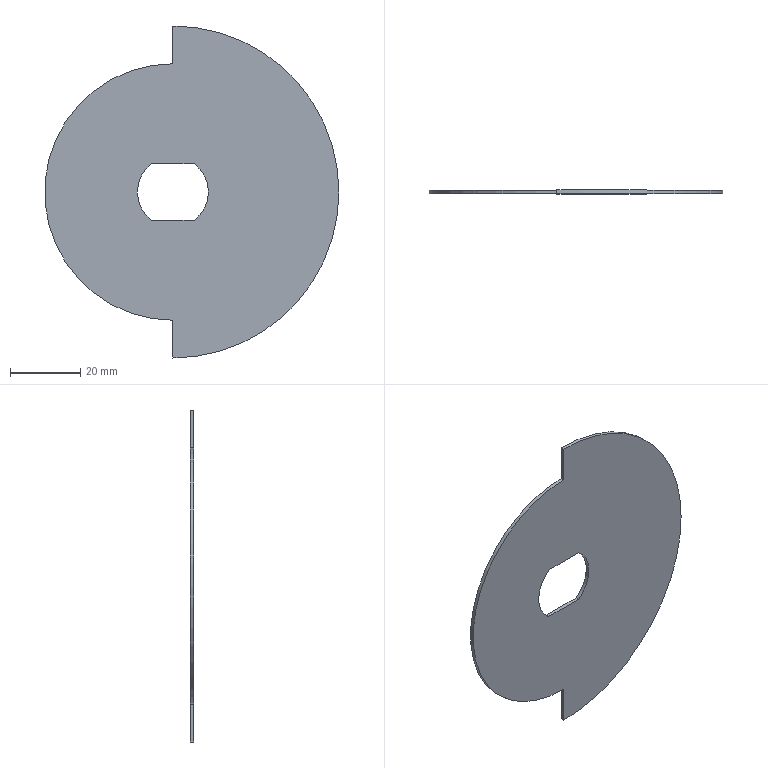Part | SolidWorks | features ICE 2, Extrusion 1 | 1 solid | 10 faces | box 83.75 x 1 x 94.5 mm | volume 5312 mm3 | plane 6 | cylinder 4 | commonest cylinder face diameters 20.2 x2 73 x1 94.5 x1
STEP:
#1=CARTESIAN_POINT('',(-6.033,1.,-8.1));
#2=VERTEX_POINT('',#1);
#3=CARTESIAN_POINT('',(-6.033,0.,-8.1));
#4=VERTEX_POINT('',#3);
#5=CARTESIAN_POINT('',(-6.033,1.,-8.1));
#6=DIRECTION('',(0.,-1.,0.));
#7=VECTOR('',#6,1000.);
#8=LINE('',#5,#7);
#9=EDGE_CURVE('',#2,#4,#8,.T.);
#10=ORIENTED_EDGE('',*,*,#9,.F.);
#11=CARTESIAN_POINT('',(-6.033,1.,8.1));
#12=VERTEX_POINT('',#11);
#13=CARTESIAN_POINT('',(0.,1.,0.));
#14=DIRECTION('',(0.,1.,0.));
#15=DIRECTION('',(0.,0.,1.));
#16=AXIS2_PLACEMENT_3D('',#13,#14,#15);
#17=CIRCLE('',#16,10.1);
#18=EDGE_CURVE('',#2,#12,#17,.T.);
#19=ORIENTED_EDGE('',*,*,#18,.T.);
#20=CARTESIAN_POINT('',(-6.033,0.,8.1));
#21=VERTEX_POINT('',#20);
#22=CARTESIAN_POINT('',(-6.033,1.,8.1));
#23=DIRECTION('',(0.,-1.,0.));
#24=VECTOR('',#23,1000.);
#25=LINE('',#22,#24);
#26=EDGE_CURVE('',#12,#21,#25,.T.);
#27=ORIENTED_EDGE('',*,*,#26,.T.);
#28=CARTESIAN_POINT('',(0.,0.,0.));
#29=DIRECTION('',(0.,1.,0.));
#30=DIRECTION('',(0.,0.,1.));
#31=AXIS2_PLACEMENT_3D('',#28,#29,#30);
#32=CIRCLE('',#31,10.1);
#33=EDGE_CURVE('',#4,#21,#32,.T.);
#34=ORIENTED_EDGE('',*,*,#33,.F.);
#35=EDGE_LOOP('',(#10,#19,#27,#34));
#36=FACE_OUTER_BOUND('',#35,.T.);
#37=CARTESIAN_POINT('',(0.,1.,0.));
#38=DIRECTION('',(0.,-1.,0.));
#39=DIRECTION('',(0.,0.,-1.));
#40=AXIS2_PLACEMENT_3D('',#37,#38,#39);
#41=CYLINDRICAL_SURFACE('',#40,10.1);
#42=ADVANCED_FACE('',(#36),#41,.F.);
#43=CARTESIAN_POINT('',(0.,1.,47.25));
#44=VERTEX_POINT('',#43);
#45=CARTESIAN_POINT('',(0.,1.,36.5));
#46=VERTEX_POINT('',#45);
#47=CARTESIAN_POINT('',(0.,1.,0.));
#48=DIRECTION('',(0.,0.,-1.));
#49=VECTOR('',#48,1000.);
#50=LINE('',#47,#49);
#51=EDGE_CURVE('',#44,#46,#50,.T.);
#52=ORIENTED_EDGE('',*,*,#51,.F.);
#53=CARTESIAN_POINT('',(0.,1.,-47.25));
#54=VERTEX_POINT('',#53);
#55=CARTESIAN_POINT('',(0.,1.,0.));
#56=DIRECTION('',(0.,1.,0.));
#57=DIRECTION('',(0.,0.,1.));
#58=AXIS2_PLACEMENT_3D('',#55,#56,#57);
#59=CIRCLE('',#58,47.25);
#60=EDGE_CURVE('',#44,#54,#59,.T.);
#61=ORIENTED_EDGE('',*,*,#60,.T.);
#62=CARTESIAN_POINT('',(0.,1.,-36.5));
#63=VERTEX_POINT('',#62);
#64=CARTESIAN_POINT('',(0.,1.,0.));
#65=DIRECTION('',(0.,0.,-1.));
#66=VECTOR('',#65,1000.);
#67=LINE('',#64,#66);
#68=EDGE_CURVE('',#63,#54,#67,.T.);
#69=ORIENTED_EDGE('',*,*,#68,.F.);
#70=CARTESIAN_POINT('',(0.,1.,0.));
#71=DIRECTION('',(0.,-1.,0.));
#72=DIRECTION('',(0.,0.,1.));
#73=AXIS2_PLACEMENT_3D('',#70,#71,#72);
#74=CIRCLE('',#73,36.5);
#75=EDGE_CURVE('',#46,#63,#74,.T.);
#76=ORIENTED_EDGE('',*,*,#75,.F.);
#77=EDGE_LOOP('',(#52,#61,#69,#76));
#78=FACE_OUTER_BOUND('',#77,.T.);
#79=CARTESIAN_POINT('',(6.033,1.,8.1));
#80=VERTEX_POINT('',#79);
#81=CARTESIAN_POINT('',(6.033,1.,-8.1));
#82=VERTEX_POINT('',#81);
#83=CARTESIAN_POINT('',(0.,1.,0.));
#84=DIRECTION('',(0.,1.,0.));
#85=DIRECTION('',(0.,0.,1.));
#86=AXIS2_PLACEMENT_3D('',#83,#84,#85);
#87=CIRCLE('',#86,10.1);
#88=EDGE_CURVE('',#80,#82,#87,.T.);
#89=ORIENTED_EDGE('',*,*,#88,.F.);
#90=CARTESIAN_POINT('',(6.033,1.,8.1));
#91=DIRECTION('',(1.,0.,0.));
#92=VECTOR('',#91,1000.);
#93=LINE('',#90,#92);
#94=EDGE_CURVE('',#12,#80,#93,.T.);
#95=ORIENTED_EDGE('',*,*,#94,.F.);
#96=ORIENTED_EDGE('',*,*,#18,.F.);
#97=CARTESIAN_POINT('',(6.033,1.,-8.1));
#98=DIRECTION('',(-1.,0.,0.));
#99=VECTOR('',#98,1000.);
#100=LINE('',#97,#99);
#101=EDGE_CURVE('',#82,#2,#100,.T.);
#102=ORIENTED_EDGE('',*,*,#101,.F.);
#103=EDGE_LOOP('',(#89,#95,#96,#102));
#104=FACE_BOUND('',#103,.T.);
#105=CARTESIAN_POINT('',(0.,1.,0.));
#106=DIRECTION('',(0.,1.,0.));
#107=DIRECTION('',(0.,0.,1.));
#108=AXIS2_PLACEMENT_3D('',#105,#106,#107);
#109=PLANE('',#108);
#110=ADVANCED_FACE('',(#78,#104),#109,.T.);
#111=CARTESIAN_POINT('',(0.,0.,47.25));
#112=VERTEX_POINT('',#111);
#113=CARTESIAN_POINT('',(0.,0.,-47.25));
#114=VERTEX_POINT('',#113);
#115=CARTESIAN_POINT('',(0.,0.,0.));
#116=DIRECTION('',(0.,1.,0.));
#117=DIRECTION('',(0.,0.,1.));
#118=AXIS2_PLACEMENT_3D('',#115,#116,#117);
#119=CIRCLE('',#118,47.25);
#120=EDGE_CURVE('',#112,#114,#119,.T.);
#121=ORIENTED_EDGE('',*,*,#120,.F.);
#122=CARTESIAN_POINT('',(0.,0.,36.5));
#123=VERTEX_POINT('',#122);
#124=CARTESIAN_POINT('',(0.,0.,47.25));
#125=DIRECTION('',(0.,0.,1.));
#126=VECTOR('',#125,1000.);
#127=LINE('',#124,#126);
#128=EDGE_CURVE('',#123,#112,#127,.T.);
#129=ORIENTED_EDGE('',*,*,#128,.F.);
#130=CARTESIAN_POINT('',(0.,0.,-36.5));
#131=VERTEX_POINT('',#130);
#132=CARTESIAN_POINT('',(0.,0.,0.));
#133=DIRECTION('',(0.,1.,0.));
#134=DIRECTION('',(0.,0.,-1.));
#135=AXIS2_PLACEMENT_3D('',#132,#133,#134);
#136=CIRCLE('',#135,36.5);
#137=EDGE_CURVE('',#131,#123,#136,.T.);
#138=ORIENTED_EDGE('',*,*,#137,.F.);
#139=CARTESIAN_POINT('',(0.,0.,-36.5));
#140=DIRECTION('',(0.,0.,1.));
#141=VECTOR('',#140,1000.);
#142=LINE('',#139,#141);
#143=EDGE_CURVE('',#114,#131,#142,.T.);
#144=ORIENTED_EDGE('',*,*,#143,.F.);
#145=EDGE_LOOP('',(#121,#129,#138,#144));
#146=FACE_OUTER_BOUND('',#145,.T.);
#147=CARTESIAN_POINT('',(6.033,0.,8.1));
#148=VERTEX_POINT('',#147);
#149=CARTESIAN_POINT('',(6.033,0.,-8.1));
#150=VERTEX_POINT('',#149);
#151=CARTESIAN_POINT('',(0.,0.,0.));
#152=DIRECTION('',(0.,1.,0.));
#153=DIRECTION('',(0.,0.,1.));
#154=AXIS2_PLACEMENT_3D('',#151,#152,#153);
#155=CIRCLE('',#154,10.1);
#156=EDGE_CURVE('',#148,#150,#155,.T.);
#157=ORIENTED_EDGE('',*,*,#156,.T.);
#158=CARTESIAN_POINT('',(6.033,0.,-8.1));
#159=DIRECTION('',(-1.,0.,0.));
#160=VECTOR('',#159,1000.);
#161=LINE('',#158,#160);
#162=EDGE_CURVE('',#150,#4,#161,.T.);
#163=ORIENTED_EDGE('',*,*,#162,.T.);
#164=ORIENTED_EDGE('',*,*,#33,.T.);
#165=CARTESIAN_POINT('',(6.033,0.,8.1));
#166=DIRECTION('',(1.,0.,0.));
#167=VECTOR('',#166,1000.);
#168=LINE('',#165,#167);
#169=EDGE_CURVE('',#21,#148,#168,.T.);
#170=ORIENTED_EDGE('',*,*,#169,.T.);
#171=EDGE_LOOP('',(#157,#163,#164,#170));
#172=FACE_BOUND('',#171,.T.);
#173=CARTESIAN_POINT('',(0.,0.,0.));
#174=DIRECTION('',(0.,1.,0.));
#175=DIRECTION('',(0.,0.,1.));
#176=AXIS2_PLACEMENT_3D('',#173,#174,#175);
#177=PLANE('',#176);
#178=ADVANCED_FACE('',(#146,#172),#177,.F.);
#179=ORIENTED_EDGE('',*,*,#60,.F.);
#180=CARTESIAN_POINT('',(0.,1.,47.25));
#181=DIRECTION('',(0.,-1.,0.));
#182=VECTOR('',#181,1000.);
#183=LINE('',#180,#182);
#184=EDGE_CURVE('',#44,#112,#183,.T.);
#185=ORIENTED_EDGE('',*,*,#184,.T.);
#186=ORIENTED_EDGE('',*,*,#120,.T.);
#187=CARTESIAN_POINT('',(0.,1.,-47.25));
#188=DIRECTION('',(0.,1.,0.));
#189=VECTOR('',#188,1000.);
#190=LINE('',#187,#189);
#191=EDGE_CURVE('',#114,#54,#190,.T.);
#192=ORIENTED_EDGE('',*,*,#191,.T.);
#193=EDGE_LOOP('',(#179,#185,#186,#192));
#194=FACE_OUTER_BOUND('',#193,.T.);
#195=CARTESIAN_POINT('',(0.,1.,0.));
#196=DIRECTION('',(0.,-1.,0.));
#197=DIRECTION('',(0.,0.,-1.));
#198=AXIS2_PLACEMENT_3D('',#195,#196,#197);
#199=CYLINDRICAL_SURFACE('',#198,47.25);
#200=ADVANCED_FACE('',(#194),#199,.T.);
#201=CARTESIAN_POINT('',(6.033,1.,-8.1));
#202=DIRECTION('',(0.,-1.,0.));
#203=VECTOR('',#202,1000.);
#204=LINE('',#201,#203);
#205=EDGE_CURVE('',#82,#150,#204,.T.);
#206=ORIENTED_EDGE('',*,*,#205,.T.);
#207=ORIENTED_EDGE('',*,*,#156,.F.);
#208=CARTESIAN_POINT('',(6.033,1.,8.1));
#209=DIRECTION('',(0.,-1.,0.));
#210=VECTOR('',#209,1000.);
#211=LINE('',#208,#210);
#212=EDGE_CURVE('',#80,#148,#211,.T.);
#213=ORIENTED_EDGE('',*,*,#212,.F.);
#214=ORIENTED_EDGE('',*,*,#88,.T.);
#215=EDGE_LOOP('',(#206,#207,#213,#214));
#216=FACE_OUTER_BOUND('',#215,.T.);
#217=CARTESIAN_POINT('',(0.,1.,0.));
#218=DIRECTION('',(0.,-1.,0.));
#219=DIRECTION('',(0.,0.,-1.));
#220=AXIS2_PLACEMENT_3D('',#217,#218,#219);
#221=CYLINDRICAL_SURFACE('',#220,10.1);
#222=ADVANCED_FACE('',(#216),#221,.F.);
#223=ORIENTED_EDGE('',*,*,#169,.F.);
#224=ORIENTED_EDGE('',*,*,#26,.F.);
#225=ORIENTED_EDGE('',*,*,#94,.T.);
#226=ORIENTED_EDGE('',*,*,#212,.T.);
#227=EDGE_LOOP('',(#223,#224,#225,#226));
#228=FACE_OUTER_BOUND('',#227,.T.);
#229=CARTESIAN_POINT('',(6.033,1.,8.1));
#230=DIRECTION('',(0.,0.,-1.));
#231=DIRECTION('',(-1.,0.,0.));
#232=AXIS2_PLACEMENT_3D('',#229,#230,#231);
#233=PLANE('',#232);
#234=ADVANCED_FACE('',(#228),#233,.T.);
#235=ORIENTED_EDGE('',*,*,#162,.F.);
#236=ORIENTED_EDGE('',*,*,#205,.F.);
#237=ORIENTED_EDGE('',*,*,#101,.T.);
#238=ORIENTED_EDGE('',*,*,#9,.T.);
#239=EDGE_LOOP('',(#235,#236,#237,#238));
#240=FACE_OUTER_BOUND('',#239,.T.);
#241=CARTESIAN_POINT('',(6.033,1.,-8.1));
#242=DIRECTION('',(0.,0.,1.));
#243=DIRECTION('',(1.,0.,0.));
#244=AXIS2_PLACEMENT_3D('',#241,#242,#243);
#245=PLANE('',#244);
#246=ADVANCED_FACE('',(#240),#245,.T.);
#247=ORIENTED_EDGE('',*,*,#51,.T.);
#248=CARTESIAN_POINT('',(0.,10.,36.5));
#249=DIRECTION('',(0.,-1.,0.));
#250=VECTOR('',#249,1000.);
#251=LINE('',#248,#250);
#252=EDGE_CURVE('',#46,#123,#251,.T.);
#253=ORIENTED_EDGE('',*,*,#252,.T.);
#254=ORIENTED_EDGE('',*,*,#128,.T.);
#255=ORIENTED_EDGE('',*,*,#184,.F.);
#256=EDGE_LOOP('',(#247,#253,#254,#255));
#257=FACE_OUTER_BOUND('',#256,.T.);
#258=CARTESIAN_POINT('',(0.,10.,47.25));
#259=DIRECTION('',(1.,0.,0.));
#260=DIRECTION('',(0.,0.,-1.));
#261=AXIS2_PLACEMENT_3D('',#258,#259,#260);
#262=PLANE('',#261);
#263=ADVANCED_FACE('',(#257),#262,.F.);
#264=ORIENTED_EDGE('',*,*,#75,.T.);
#265=CARTESIAN_POINT('',(0.,10.,-36.5));
#266=DIRECTION('',(0.,-1.,0.));
#267=VECTOR('',#266,1000.);
#268=LINE('',#265,#267);
#269=EDGE_CURVE('',#63,#131,#268,.T.);
#270=ORIENTED_EDGE('',*,*,#269,.T.);
#271=ORIENTED_EDGE('',*,*,#137,.T.);
#272=ORIENTED_EDGE('',*,*,#252,.F.);
#273=EDGE_LOOP('',(#264,#270,#271,#272));
#274=FACE_OUTER_BOUND('',#273,.T.);
#275=CARTESIAN_POINT('',(0.,10.,0.));
#276=DIRECTION('',(0.,-1.,0.));
#277=DIRECTION('',(0.,0.,-1.));
#278=AXIS2_PLACEMENT_3D('',#275,#276,#277);
#279=CYLINDRICAL_SURFACE('',#278,36.5);
#280=ADVANCED_FACE('',(#274),#279,.T.);
#281=ORIENTED_EDGE('',*,*,#68,.T.);
#282=ORIENTED_EDGE('',*,*,#191,.F.);
#283=ORIENTED_EDGE('',*,*,#143,.T.);
#284=ORIENTED_EDGE('',*,*,#269,.F.);
#285=EDGE_LOOP('',(#281,#282,#283,#284));
#286=FACE_OUTER_BOUND('',#285,.T.);
#287=CARTESIAN_POINT('',(0.,10.,-36.5));
#288=DIRECTION('',(1.,0.,0.));
#289=DIRECTION('',(0.,0.,-1.));
#290=AXIS2_PLACEMENT_3D('',#287,#288,#289);
#291=PLANE('',#290);
#292=ADVANCED_FACE('',(#286),#291,.F.);
#293=CLOSED_SHELL('',(#42,#110,#178,#200,#222,#234,#246,#263,#280,#292));
#294=MANIFOLD_SOLID_BREP('',#293);
#295=CARTESIAN_POINT('',(0.,0.,0.));
#296=DIRECTION('',(0.,0.,1.));
#297=DIRECTION('',(1.,0.,0.));
#298=AXIS2_PLACEMENT_3D('',#295,#296,#297);
#299=(LENGTH_UNIT()NAMED_UNIT(*)SI_UNIT(.MILLI.,.METRE.));
#300=UNCERTAINTY_MEASURE_WITH_UNIT(LENGTH_MEASURE(0.00001),#299,'','');
#301=(NAMED_UNIT(*)PLANE_ANGLE_UNIT()SI_UNIT($,.RADIAN.));
#302=(NAMED_UNIT(*)SI_UNIT($,.STERADIAN.)SOLID_ANGLE_UNIT());
#303=(GEOMETRIC_REPRESENTATION_CONTEXT(3)GLOBAL_UNCERTAINTY_ASSIGNED_CONTEXT((#300))GLOBAL_UNIT_ASSIGNED_CONTEXT((#299,#301,#302))REPRESENTATION_CONTEXT('',''));
#304=ADVANCED_BREP_SHAPE_REPRESENTATION('',(#294,#298),#303);